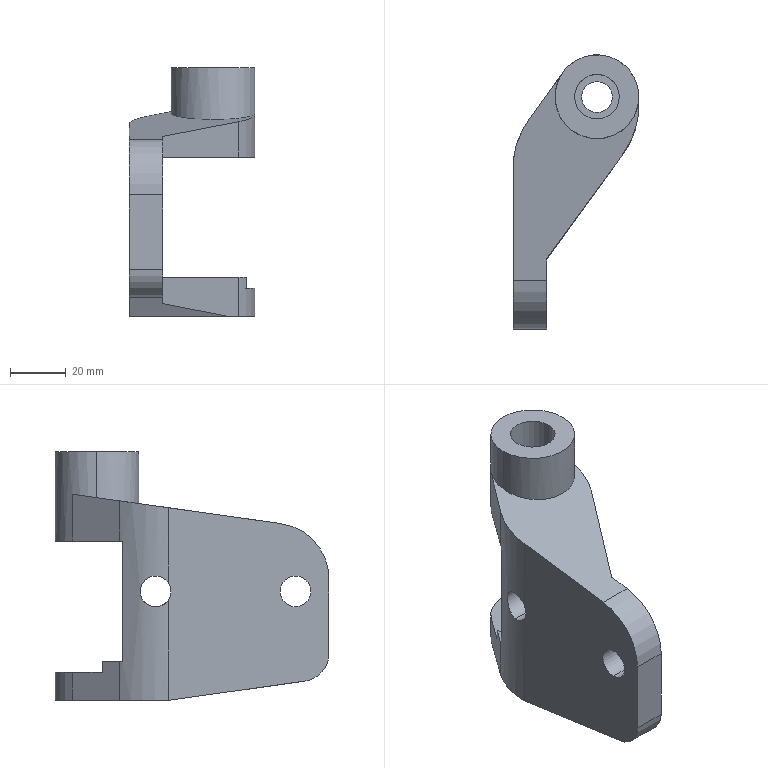Part | SolidWorks | features BaseBody 1 | 1 solid | 40 faces | box 45 x 98 x 89 mm | volume 93140 mm3 | cylinder 21 | plane 19 | commonest cylinder face diameters 11 x6 20 x5 30 x3 60 x3 16 x2 40 x2
STEP:
#1=CARTESIAN_POINT('',(-30.,-71.,33.5));
#2=VERTEX_POINT('',#1);
#3=CARTESIAN_POINT('',(-30.,-71.,44.5));
#4=VERTEX_POINT('',#3);
#5=CARTESIAN_POINT('',(-30.,-71.,39.));
#6=DIRECTION('',(-1.,0.,0.));
#7=DIRECTION('',(0.,0.,-1.));
#8=AXIS2_PLACEMENT_3D('',#5,#6,#7);
#9=CIRCLE('',#8,5.5);
#10=EDGE_CURVE('',#2,#4,#9,.T.);
#11=ORIENTED_EDGE('',*,*,#10,.T.);
#12=CARTESIAN_POINT('',(-19.,-71.,44.5));
#13=VERTEX_POINT('',#12);
#14=CARTESIAN_POINT('',(-30.,-71.,44.5));
#15=DIRECTION('',(1.,0.,0.));
#16=VECTOR('',#15,1000.);
#17=LINE('',#14,#16);
#18=EDGE_CURVE('',#4,#13,#17,.T.);
#19=ORIENTED_EDGE('',*,*,#18,.T.);
#20=CARTESIAN_POINT('',(-19.,-71.,33.5));
#21=VERTEX_POINT('',#20);
#22=CARTESIAN_POINT('',(-19.,-71.,39.));
#23=DIRECTION('',(-1.,0.,0.));
#24=DIRECTION('',(0.,0.,-1.));
#25=AXIS2_PLACEMENT_3D('',#22,#23,#24);
#26=CIRCLE('',#25,5.5);
#27=EDGE_CURVE('',#21,#13,#26,.T.);
#28=ORIENTED_EDGE('',*,*,#27,.F.);
#29=CARTESIAN_POINT('',(-30.,-71.,33.5));
#30=DIRECTION('',(1.,0.,0.));
#31=VECTOR('',#30,1000.);
#32=LINE('',#29,#31);
#33=EDGE_CURVE('',#2,#21,#32,.T.);
#34=ORIENTED_EDGE('',*,*,#33,.F.);
#35=EDGE_LOOP('',(#11,#19,#28,#34));
#36=FACE_OUTER_BOUND('',#35,.T.);
#37=CARTESIAN_POINT('',(-30.,-71.,39.));
#38=DIRECTION('',(1.,0.,0.));
#39=DIRECTION('',(0.,0.,-1.));
#40=AXIS2_PLACEMENT_3D('',#37,#38,#39);
#41=CYLINDRICAL_SURFACE('',#40,5.5);
#42=ADVANCED_FACE('',(#36),#41,.F.);
#43=CARTESIAN_POINT('',(-29.641,-21.,44.5));
#44=VERTEX_POINT('',#43);
#45=CARTESIAN_POINT('',(-30.,-25.63,41.969));
#46=VERTEX_POINT('',#45);
#47=CARTESIAN_POINT('',(-29.641,-21.,44.5));
#48=CARTESIAN_POINT('',(-29.676,-21.226,44.5));
#49=CARTESIAN_POINT('',(-29.709,-21.456,44.486));
#50=CARTESIAN_POINT('',(-29.769,-21.91,44.429));
#51=CARTESIAN_POINT('',(-29.796,-22.134,44.387));
#52=CARTESIAN_POINT('',(-29.845,-22.574,44.275));
#53=CARTESIAN_POINT('',(-29.866,-22.791,44.205));
#54=CARTESIAN_POINT('',(-29.904,-23.218,44.038));
#55=CARTESIAN_POINT('',(-29.92,-23.429,43.94));
#56=CARTESIAN_POINT('',(-29.96,-24.033,43.611));
#57=CARTESIAN_POINT('',(-29.977,-24.405,43.344));
#58=CARTESIAN_POINT('',(-29.997,-25.082,42.715));
#59=CARTESIAN_POINT('',(-30.,-25.379,42.36));
#60=CARTESIAN_POINT('',(-30.,-25.63,41.969));
#61=B_SPLINE_CURVE_WITH_KNOTS('',3,(#47,#48,#49,#50,#51,#52,#53,#54,#55,#56,#57,#58,#59,#60),.UNSPECIFIED.,.F.,.F.,(4,2,2,2,2,2,4),(0.008728,0.009414,0.0101,0.01079,0.01147,0.01284,0.01422),.UNSPECIFIED.);
#62=EDGE_CURVE('',#44,#46,#61,.T.);
#63=ORIENTED_EDGE('',*,*,#62,.F.);
#64=CARTESIAN_POINT('',(-19.,-21.,44.5));
#65=VERTEX_POINT('',#64);
#66=CARTESIAN_POINT('',(-30.,-21.,44.5));
#67=DIRECTION('',(1.,0.,0.));
#68=VECTOR('',#67,1000.);
#69=LINE('',#66,#68);
#70=EDGE_CURVE('',#44,#65,#69,.T.);
#71=ORIENTED_EDGE('',*,*,#70,.T.);
#72=CARTESIAN_POINT('',(-19.,-21.,33.5));
#73=VERTEX_POINT('',#72);
#74=CARTESIAN_POINT('',(-19.,-21.,39.));
#75=DIRECTION('',(-1.,0.,0.));
#76=DIRECTION('',(0.,0.,-1.));
#77=AXIS2_PLACEMENT_3D('',#74,#75,#76);
#78=CIRCLE('',#77,5.5);
#79=EDGE_CURVE('',#73,#65,#78,.T.);
#80=ORIENTED_EDGE('',*,*,#79,.F.);
#81=CARTESIAN_POINT('',(-29.641,-21.,33.5));
#82=VERTEX_POINT('',#81);
#83=CARTESIAN_POINT('',(-30.,-21.,33.5));
#84=DIRECTION('',(1.,0.,0.));
#85=VECTOR('',#84,1000.);
#86=LINE('',#83,#85);
#87=EDGE_CURVE('',#82,#73,#86,.T.);
#88=ORIENTED_EDGE('',*,*,#87,.F.);
#89=CARTESIAN_POINT('',(-30.,-25.63,36.031));
#90=VERTEX_POINT('',#89);
#91=CARTESIAN_POINT('',(-30.,-25.63,36.031));
#92=CARTESIAN_POINT('',(-30.,-25.379,35.64));
#93=CARTESIAN_POINT('',(-29.997,-25.085,35.289));
#94=CARTESIAN_POINT('',(-29.982,-24.581,34.819));
#95=CARTESIAN_POINT('',(-29.975,-24.401,34.671));
#96=CARTESIAN_POINT('',(-29.958,-24.026,34.402));
#97=CARTESIAN_POINT('',(-29.947,-23.832,34.28));
#98=CARTESIAN_POINT('',(-29.92,-23.431,34.061));
#99=CARTESIAN_POINT('',(-29.904,-23.223,33.964));
#100=CARTESIAN_POINT('',(-29.867,-22.795,33.796));
#101=CARTESIAN_POINT('',(-29.845,-22.574,33.725));
#102=CARTESIAN_POINT('',(-29.772,-21.91,33.557));
#103=CARTESIAN_POINT('',(-29.712,-21.459,33.5));
#104=CARTESIAN_POINT('',(-29.641,-21.,33.5));
#105=B_SPLINE_CURVE_WITH_KNOTS('',3,(#91,#92,#93,#94,#95,#96,#97,#98,#99,#100,#101,#102,#103,#104),.UNSPECIFIED.,.F.,.F.,(4,2,2,2,2,2,4),(-0.01422,-0.01284,-0.01216,-0.01147,-0.01078,-0.0101,-0.008723),.UNSPECIFIED.);
#106=EDGE_CURVE('',#90,#82,#105,.T.);
#107=ORIENTED_EDGE('',*,*,#106,.F.);
#108=CARTESIAN_POINT('',(-30.,-21.,39.));
#109=DIRECTION('',(-1.,0.,0.));
#110=DIRECTION('',(0.,0.,-1.));
#111=AXIS2_PLACEMENT_3D('',#108,#109,#110);
#112=CIRCLE('',#111,5.5);
#113=EDGE_CURVE('',#90,#46,#112,.T.);
#114=ORIENTED_EDGE('',*,*,#113,.T.);
#115=EDGE_LOOP('',(#63,#71,#80,#88,#107,#114));
#116=FACE_OUTER_BOUND('',#115,.T.);
#117=CARTESIAN_POINT('',(-30.,-21.,39.));
#118=DIRECTION('',(1.,0.,0.));
#119=DIRECTION('',(0.,0.,-1.));
#120=AXIS2_PLACEMENT_3D('',#117,#118,#119);
#121=CYLINDRICAL_SURFACE('',#120,5.5);
#122=ADVANCED_FACE('',(#116),#121,.F.);
#123=CARTESIAN_POINT('',(-15.,0.,89.));
#124=VERTEX_POINT('',#123);
#125=CARTESIAN_POINT('',(15.,0.,89.));
#126=VERTEX_POINT('',#125);
#127=CARTESIAN_POINT('',(0.,0.,89.));
#128=DIRECTION('',(0.,0.,-1.));
#129=DIRECTION('',(-1.,0.,0.));
#130=AXIS2_PLACEMENT_3D('',#127,#128,#129);
#131=CIRCLE('',#130,15.);
#132=EDGE_CURVE('',#124,#126,#131,.T.);
#133=ORIENTED_EDGE('',*,*,#132,.T.);
#134=CARTESIAN_POINT('',(15.,-0.000000405,72.514));
#135=VERTEX_POINT('',#134);
#136=CARTESIAN_POINT('',(15.,0.,89.));
#137=DIRECTION('',(0.,0.,-1.));
#138=VECTOR('',#137,1000.);
#139=LINE('',#136,#138);
#140=EDGE_CURVE('',#126,#135,#139,.T.);
#141=ORIENTED_EDGE('',*,*,#140,.T.);
#142=CARTESIAN_POINT('',(15.,-0.000000405,57.));
#143=VERTEX_POINT('',#142);
#144=CARTESIAN_POINT('',(15.,-0.00000081,89.));
#145=DIRECTION('',(0.,0.,-1.));
#146=VECTOR('',#145,1000.);
#147=LINE('',#144,#146);
#148=EDGE_CURVE('',#135,#143,#147,.T.);
#149=ORIENTED_EDGE('',*,*,#148,.T.);
#150=CARTESIAN_POINT('',(-12.163,8.779,57.));
#151=VERTEX_POINT('',#150);
#152=CARTESIAN_POINT('',(0.,0.,57.));
#153=DIRECTION('',(0.,0.,1.));
#154=DIRECTION('',(-1.,0.,0.));
#155=AXIS2_PLACEMENT_3D('',#152,#153,#154);
#156=CIRCLE('',#155,15.);
#157=EDGE_CURVE('',#143,#151,#156,.T.);
#158=ORIENTED_EDGE('',*,*,#157,.T.);
#159=CARTESIAN_POINT('',(-12.163,8.779,73.747));
#160=VERTEX_POINT('',#159);
#161=CARTESIAN_POINT('',(-12.163,8.779,65.374));
#162=DIRECTION('',(0.,0.,1.));
#163=VECTOR('',#162,1000.);
#164=LINE('',#161,#163);
#165=EDGE_CURVE('',#151,#160,#164,.T.);
#166=ORIENTED_EDGE('',*,*,#165,.T.);
#167=CARTESIAN_POINT('',(-15.,0.,72.514));
#168=VERTEX_POINT('',#167);
#169=CARTESIAN_POINT('',(-15.,0.,72.514));
#170=CARTESIAN_POINT('',(-15.,3.178,72.96));
#171=CARTESIAN_POINT('',(-14.023,6.202,73.385));
#172=CARTESIAN_POINT('',(-12.163,8.779,73.747));
#173=(BOUNDED_CURVE()B_SPLINE_CURVE(3,(#169,#170,#171,#172),.UNSPECIFIED.,.F.,.F.)B_SPLINE_CURVE_WITH_KNOTS((4,4),(1.571,2.196),.UNSPECIFIED.)CURVE()GEOMETRIC_REPRESENTATION_ITEM()RATIONAL_B_SPLINE_CURVE((1.,0.9677,0.9677,1.))REPRESENTATION_ITEM(''));
#174=EDGE_CURVE('',#168,#160,#173,.T.);
#175=ORIENTED_EDGE('',*,*,#174,.F.);
#176=CARTESIAN_POINT('',(-15.,0.,89.));
#177=DIRECTION('',(0.,0.,-1.));
#178=VECTOR('',#177,1000.);
#179=LINE('',#176,#178);
#180=EDGE_CURVE('',#124,#168,#179,.T.);
#181=ORIENTED_EDGE('',*,*,#180,.F.);
#182=EDGE_LOOP('',(#133,#141,#149,#158,#166,#175,#181));
#183=FACE_OUTER_BOUND('',#182,.T.);
#184=CARTESIAN_POINT('',(0.,0.,89.));
#185=DIRECTION('',(0.,0.,-1.));
#186=DIRECTION('',(-1.,0.,0.));
#187=AXIS2_PLACEMENT_3D('',#184,#185,#186);
#188=CYLINDRICAL_SURFACE('',#187,15.);
#189=ADVANCED_FACE('',(#183),#188,.T.);
#190=CARTESIAN_POINT('',(-18.,-71.,29.));
#191=VERTEX_POINT('',#190);
#192=CARTESIAN_POINT('',(-18.,-71.,49.));
#193=VERTEX_POINT('',#192);
#194=CARTESIAN_POINT('',(-18.,-71.,39.));
#195=DIRECTION('',(-1.,0.,0.));
#196=DIRECTION('',(0.,0.,1.));
#197=AXIS2_PLACEMENT_3D('',#194,#195,#196);
#198=CIRCLE('',#197,10.);
#199=EDGE_CURVE('',#191,#193,#198,.T.);
#200=ORIENTED_EDGE('',*,*,#199,.F.);
#201=CARTESIAN_POINT('',(-19.,-71.,29.));
#202=VERTEX_POINT('',#201);
#203=CARTESIAN_POINT('',(-18.,-71.,29.));
#204=DIRECTION('',(-1.,0.,0.));
#205=VECTOR('',#204,1000.);
#206=LINE('',#203,#205);
#207=EDGE_CURVE('',#191,#202,#206,.T.);
#208=ORIENTED_EDGE('',*,*,#207,.T.);
#209=CARTESIAN_POINT('',(-19.,-71.,49.));
#210=VERTEX_POINT('',#209);
#211=CARTESIAN_POINT('',(-19.,-71.,39.));
#212=DIRECTION('',(1.,0.,0.));
#213=DIRECTION('',(0.,0.,1.));
#214=AXIS2_PLACEMENT_3D('',#211,#212,#213);
#215=CIRCLE('',#214,10.);
#216=EDGE_CURVE('',#210,#202,#215,.T.);
#217=ORIENTED_EDGE('',*,*,#216,.F.);
#218=CARTESIAN_POINT('',(-18.,-71.,49.));
#219=DIRECTION('',(-1.,0.,0.));
#220=VECTOR('',#219,1000.);
#221=LINE('',#218,#220);
#222=EDGE_CURVE('',#193,#210,#221,.T.);
#223=ORIENTED_EDGE('',*,*,#222,.F.);
#224=EDGE_LOOP('',(#200,#208,#217,#223));
#225=FACE_OUTER_BOUND('',#224,.T.);
#226=CARTESIAN_POINT('',(-18.,-71.,39.));
#227=DIRECTION('',(-1.,0.,0.));
#228=DIRECTION('',(0.,0.,1.));
#229=AXIS2_PLACEMENT_3D('',#226,#227,#228);
#230=CYLINDRICAL_SURFACE('',#229,10.);
#231=ADVANCED_FACE('',(#225),#230,.F.);
#232=CARTESIAN_POINT('',(-18.,-21.,29.));
#233=VERTEX_POINT('',#232);
#234=CARTESIAN_POINT('',(-18.,-21.,49.));
#235=VERTEX_POINT('',#234);
#236=CARTESIAN_POINT('',(-18.,-21.,39.));
#237=DIRECTION('',(-1.,0.,0.));
#238=DIRECTION('',(0.,0.,1.));
#239=AXIS2_PLACEMENT_3D('',#236,#237,#238);
#240=CIRCLE('',#239,10.);
#241=EDGE_CURVE('',#233,#235,#240,.T.);
#242=ORIENTED_EDGE('',*,*,#241,.F.);
#243=CARTESIAN_POINT('',(-19.,-21.,29.));
#244=VERTEX_POINT('',#243);
#245=CARTESIAN_POINT('',(-18.,-21.,29.));
#246=DIRECTION('',(-1.,0.,0.));
#247=VECTOR('',#246,1000.);
#248=LINE('',#245,#247);
#249=EDGE_CURVE('',#233,#244,#248,.T.);
#250=ORIENTED_EDGE('',*,*,#249,.T.);
#251=CARTESIAN_POINT('',(-19.,-21.,49.));
#252=VERTEX_POINT('',#251);
#253=CARTESIAN_POINT('',(-19.,-21.,39.));
#254=DIRECTION('',(1.,0.,0.));
#255=DIRECTION('',(0.,0.,1.));
#256=AXIS2_PLACEMENT_3D('',#253,#254,#255);
#257=CIRCLE('',#256,10.);
#258=EDGE_CURVE('',#252,#244,#257,.T.);
#259=ORIENTED_EDGE('',*,*,#258,.F.);
#260=CARTESIAN_POINT('',(-18.,-21.,49.));
#261=DIRECTION('',(-1.,0.,0.));
#262=VECTOR('',#261,1000.);
#263=LINE('',#260,#262);
#264=EDGE_CURVE('',#235,#252,#263,.T.);
#265=ORIENTED_EDGE('',*,*,#264,.F.);
#266=EDGE_LOOP('',(#242,#250,#259,#265));
#267=FACE_OUTER_BOUND('',#266,.T.);
#268=CARTESIAN_POINT('',(-18.,-21.,39.));
#269=DIRECTION('',(-1.,0.,0.));
#270=DIRECTION('',(0.,0.,1.));
#271=AXIS2_PLACEMENT_3D('',#268,#269,#270);
#272=CYLINDRICAL_SURFACE('',#271,10.);
#273=ADVANCED_FACE('',(#267),#272,.F.);
#274=CARTESIAN_POINT('',(5.5,0.,0.));
#275=VERTEX_POINT('',#274);
#276=CARTESIAN_POINT('',(-5.5,0.,0.));
#277=VERTEX_POINT('',#276);
#278=CARTESIAN_POINT('',(0.,0.,0.));
#279=DIRECTION('',(0.,0.,-1.));
#280=DIRECTION('',(1.,0.,0.));
#281=AXIS2_PLACEMENT_3D('',#278,#279,#280);
#282=CIRCLE('',#281,5.5);
#283=EDGE_CURVE('',#275,#277,#282,.T.);
#284=ORIENTED_EDGE('',*,*,#283,.T.);
#285=CARTESIAN_POINT('',(-5.5,0.,10.));
#286=VERTEX_POINT('',#285);
#287=CARTESIAN_POINT('',(-5.5,0.,0.));
#288=DIRECTION('',(0.,0.,1.));
#289=VECTOR('',#288,1000.);
#290=LINE('',#287,#289);
#291=EDGE_CURVE('',#277,#286,#290,.T.);
#292=ORIENTED_EDGE('',*,*,#291,.T.);
#293=CARTESIAN_POINT('',(5.5,0.,10.));
#294=VERTEX_POINT('',#293);
#295=CARTESIAN_POINT('',(0.,0.,10.));
#296=DIRECTION('',(0.,0.,-1.));
#297=DIRECTION('',(1.,0.,0.));
#298=AXIS2_PLACEMENT_3D('',#295,#296,#297);
#299=CIRCLE('',#298,5.5);
#300=EDGE_CURVE('',#294,#286,#299,.T.);
#301=ORIENTED_EDGE('',*,*,#300,.F.);
#302=CARTESIAN_POINT('',(5.5,0.,0.));
#303=DIRECTION('',(0.,0.,1.));
#304=VECTOR('',#303,1000.);
#305=LINE('',#302,#304);
#306=EDGE_CURVE('',#275,#294,#305,.T.);
#307=ORIENTED_EDGE('',*,*,#306,.F.);
#308=EDGE_LOOP('',(#284,#292,#301,#307));
#309=FACE_OUTER_BOUND('',#308,.T.);
#310=CARTESIAN_POINT('',(0.,0.,0.));
#311=DIRECTION('',(0.,0.,1.));
#312=DIRECTION('',(1.,0.,0.));
#313=AXIS2_PLACEMENT_3D('',#310,#311,#312);
#314=CYLINDRICAL_SURFACE('',#313,5.5);
#315=ADVANCED_FACE('',(#309),#314,.F.);
#316=CARTESIAN_POINT('',(8.,0.,89.));
#317=VERTEX_POINT('',#316);
#318=CARTESIAN_POINT('',(-8.,0.,89.));
#319=VERTEX_POINT('',#318);
#320=CARTESIAN_POINT('',(0.,0.,89.));
#321=DIRECTION('',(0.,0.,-1.));
#322=DIRECTION('',(-1.,0.,0.));
#323=AXIS2_PLACEMENT_3D('',#320,#321,#322);
#324=CIRCLE('',#323,8.);
#325=EDGE_CURVE('',#317,#319,#324,.T.);
#326=ORIENTED_EDGE('',*,*,#325,.F.);
#327=CARTESIAN_POINT('',(8.,0.,57.));
#328=VERTEX_POINT('',#327);
#329=CARTESIAN_POINT('',(8.,0.,89.));
#330=DIRECTION('',(0.,0.,-1.));
#331=VECTOR('',#330,1000.);
#332=LINE('',#329,#331);
#333=EDGE_CURVE('',#317,#328,#332,.T.);
#334=ORIENTED_EDGE('',*,*,#333,.T.);
#335=CARTESIAN_POINT('',(-8.,0.,57.));
#336=VERTEX_POINT('',#335);
#337=CARTESIAN_POINT('',(0.,0.,57.));
#338=DIRECTION('',(0.,0.,-1.));
#339=DIRECTION('',(-1.,0.,0.));
#340=AXIS2_PLACEMENT_3D('',#337,#338,#339);
#341=CIRCLE('',#340,8.);
#342=EDGE_CURVE('',#328,#336,#341,.T.);
#343=ORIENTED_EDGE('',*,*,#342,.T.);
#344=CARTESIAN_POINT('',(-8.,0.,89.));
#345=DIRECTION('',(0.,0.,-1.));
#346=VECTOR('',#345,1000.);
#347=LINE('',#344,#346);
#348=EDGE_CURVE('',#319,#336,#347,.T.);
#349=ORIENTED_EDGE('',*,*,#348,.F.);
#350=EDGE_LOOP('',(#326,#334,#343,#349));
#351=FACE_OUTER_BOUND('',#350,.T.);
#352=CARTESIAN_POINT('',(0.,0.,89.));
#353=DIRECTION('',(0.,0.,-1.));
#354=DIRECTION('',(-1.,0.,0.));
#355=AXIS2_PLACEMENT_3D('',#352,#353,#354);
#356=CYLINDRICAL_SURFACE('',#355,8.);
#357=ADVANCED_FACE('',(#351),#356,.F.);
#358=ORIENTED_EDGE('',*,*,#10,.F.);
#359=CARTESIAN_POINT('',(-30.,-71.,39.));
#360=DIRECTION('',(-1.,0.,0.));
#361=DIRECTION('',(0.,0.,-1.));
#362=AXIS2_PLACEMENT_3D('',#359,#360,#361);
#363=CIRCLE('',#362,5.5);
#364=EDGE_CURVE('',#4,#2,#363,.T.);
#365=ORIENTED_EDGE('',*,*,#364,.F.);
#366=EDGE_LOOP('',(#358,#365));
#367=FACE_BOUND('',#366,.T.);
#368=CARTESIAN_POINT('',(-30.,-25.63,68.911));
#369=VERTEX_POINT('',#368);
#370=CARTESIAN_POINT('',(-30.,-65.783,63.268));
#371=VERTEX_POINT('',#370);
#372=CARTESIAN_POINT('',(-30.,-25.63,68.911));
#373=DIRECTION('',(0.,-0.9903,-0.1392));
#374=VECTOR('',#373,1000.);
#375=LINE('',#372,#374);
#376=EDGE_CURVE('',#369,#371,#375,.T.);
#377=ORIENTED_EDGE('',*,*,#376,.F.);
#378=CARTESIAN_POINT('',(-30.,-25.63,34.475));
#379=DIRECTION('',(0.,0.,1.));
#380=VECTOR('',#379,1000.);
#381=LINE('',#378,#380);
#382=EDGE_CURVE('',#46,#369,#381,.T.);
#383=ORIENTED_EDGE('',*,*,#382,.F.);
#384=ORIENTED_EDGE('',*,*,#113,.F.);
#385=CARTESIAN_POINT('',(-30.,-25.63,0.03827));
#386=VERTEX_POINT('',#385);
#387=CARTESIAN_POINT('',(-30.,-25.63,34.475));
#388=DIRECTION('',(0.,0.,1.));
#389=VECTOR('',#388,1000.);
#390=LINE('',#387,#389);
#391=EDGE_CURVE('',#386,#90,#390,.T.);
#392=ORIENTED_EDGE('',*,*,#391,.F.);
#393=CARTESIAN_POINT('',(-30.,-74.392,6.891));
#394=VERTEX_POINT('',#393);
#395=CARTESIAN_POINT('',(-30.,-74.392,6.891));
#396=DIRECTION('',(0.,0.9903,-0.1392));
#397=VECTOR('',#396,1000.);
#398=LINE('',#395,#397);
#399=EDGE_CURVE('',#394,#386,#398,.T.);
#400=ORIENTED_EDGE('',*,*,#399,.F.);
#401=CARTESIAN_POINT('',(-30.,-83.,16.794));
#402=VERTEX_POINT('',#401);
#403=CARTESIAN_POINT('',(-30.,-73.,16.794));
#404=DIRECTION('',(1.,0.,0.));
#405=DIRECTION('',(0.,0.,1.));
#406=AXIS2_PLACEMENT_3D('',#403,#404,#405);
#407=CIRCLE('',#406,10.);
#408=EDGE_CURVE('',#402,#394,#407,.T.);
#409=ORIENTED_EDGE('',*,*,#408,.F.);
#410=CARTESIAN_POINT('',(-30.,-83.,43.463));
#411=VERTEX_POINT('',#410);
#412=CARTESIAN_POINT('',(-30.,-83.,34.475));
#413=DIRECTION('',(0.,0.,-1.));
#414=VECTOR('',#413,1000.);
#415=LINE('',#412,#414);
#416=EDGE_CURVE('',#411,#402,#415,.T.);
#417=ORIENTED_EDGE('',*,*,#416,.F.);
#418=CARTESIAN_POINT('',(-30.,-63.,43.463));
#419=DIRECTION('',(1.,0.,0.));
#420=DIRECTION('',(0.,0.,1.));
#421=AXIS2_PLACEMENT_3D('',#418,#419,#420);
#422=CIRCLE('',#421,20.);
#423=EDGE_CURVE('',#371,#411,#422,.T.);
#424=ORIENTED_EDGE('',*,*,#423,.F.);
#425=EDGE_LOOP('',(#377,#383,#384,#392,#400,#409,#417,#424));
#426=FACE_OUTER_BOUND('',#425,.T.);
#427=CARTESIAN_POINT('',(-30.,-54.315,34.475));
#428=DIRECTION('',(1.,0.,0.));
#429=DIRECTION('',(0.,0.,-1.));
#430=AXIS2_PLACEMENT_3D('',#427,#428,#429);
#431=PLANE('',#430);
#432=ADVANCED_FACE('',(#367,#426),#431,.F.);
#433=ORIENTED_EDGE('',*,*,#18,.F.);
#434=ORIENTED_EDGE('',*,*,#364,.T.);
#435=ORIENTED_EDGE('',*,*,#33,.T.);
#436=CARTESIAN_POINT('',(-19.,-71.,39.));
#437=DIRECTION('',(-1.,0.,0.));
#438=DIRECTION('',(0.,0.,-1.));
#439=AXIS2_PLACEMENT_3D('',#436,#437,#438);
#440=CIRCLE('',#439,5.5);
#441=EDGE_CURVE('',#13,#21,#440,.T.);
#442=ORIENTED_EDGE('',*,*,#441,.F.);
#443=EDGE_LOOP('',(#433,#434,#435,#442));
#444=FACE_OUTER_BOUND('',#443,.T.);
#445=CARTESIAN_POINT('',(-30.,-71.,39.));
#446=DIRECTION('',(1.,0.,0.));
#447=DIRECTION('',(0.,0.,-1.));
#448=AXIS2_PLACEMENT_3D('',#445,#446,#447);
#449=CYLINDRICAL_SURFACE('',#448,5.5);
#450=ADVANCED_FACE('',(#444),#449,.F.);
#451=CARTESIAN_POINT('',(-18.,-83.,43.463));
#452=VERTEX_POINT('',#451);
#453=CARTESIAN_POINT('',(-18.,-83.,43.463));
#454=DIRECTION('',(1.,0.,0.));
#455=VECTOR('',#454,1000.);
#456=LINE('',#453,#455);
#457=EDGE_CURVE('',#411,#452,#456,.T.);
#458=ORIENTED_EDGE('',*,*,#457,.T.);
#459=CARTESIAN_POINT('',(-18.,-65.783,63.268));
#460=VERTEX_POINT('',#459);
#461=CARTESIAN_POINT('',(-18.,-63.,43.463));
#462=DIRECTION('',(-1.,0.,0.));
#463=DIRECTION('',(0.,0.,1.));
#464=AXIS2_PLACEMENT_3D('',#461,#462,#463);
#465=CIRCLE('',#464,20.);
#466=EDGE_CURVE('',#452,#460,#465,.T.);
#467=ORIENTED_EDGE('',*,*,#466,.T.);
#468=CARTESIAN_POINT('',(-18.,-65.783,63.268));
#469=DIRECTION('',(-1.,0.,0.));
#470=VECTOR('',#469,1000.);
#471=LINE('',#468,#470);
#472=EDGE_CURVE('',#460,#371,#471,.T.);
#473=ORIENTED_EDGE('',*,*,#472,.T.);
#474=ORIENTED_EDGE('',*,*,#423,.T.);
#475=EDGE_LOOP('',(#458,#467,#473,#474));
#476=FACE_OUTER_BOUND('',#475,.T.);
#477=CARTESIAN_POINT('',(-18.,-63.,43.463));
#478=DIRECTION('',(-1.,0.,0.));
#479=DIRECTION('',(0.,0.,1.));
#480=AXIS2_PLACEMENT_3D('',#477,#478,#479);
#481=CYLINDRICAL_SURFACE('',#480,20.);
#482=ADVANCED_FACE('',(#476),#481,.T.);
#483=CARTESIAN_POINT('',(15.,-0.000000405,72.514));
#484=CARTESIAN_POINT('',(15.,-30.,68.297));
#485=CARTESIAN_POINT('',(-15.,-30.,68.297));
#486=CARTESIAN_POINT('',(-15.,0.,72.514));
#487=(BOUNDED_CURVE()B_SPLINE_CURVE(3,(#483,#484,#485,#486),.UNSPECIFIED.,.F.,.F.)B_SPLINE_CURVE_WITH_KNOTS((4,4),(4.712,7.854),.UNSPECIFIED.)CURVE()GEOMETRIC_REPRESENTATION_ITEM()RATIONAL_B_SPLINE_CURVE((1.,0.3333,0.3333,1.))REPRESENTATION_ITEM(''));
#488=EDGE_CURVE('',#135,#168,#487,.T.);
#489=ORIENTED_EDGE('',*,*,#488,.T.);
#490=ORIENTED_EDGE('',*,*,#174,.T.);
#491=CARTESIAN_POINT('',(-24.325,-8.072,71.379));
#492=VERTEX_POINT('',#491);
#493=CARTESIAN_POINT('',(-12.163,8.779,73.747));
#494=DIRECTION('',(-0.5815,-0.8056,-0.1132));
#495=VECTOR('',#494,1000.);
#496=LINE('',#493,#495);
#497=EDGE_CURVE('',#160,#492,#496,.T.);
#498=ORIENTED_EDGE('',*,*,#497,.T.);
#499=CARTESIAN_POINT('',(-24.325,-8.072,71.379));
#500=CARTESIAN_POINT('',(-28.045,-13.226,70.655));
#501=CARTESIAN_POINT('',(-30.,-19.274,69.805));
#502=CARTESIAN_POINT('',(-30.,-25.63,68.911));
#503=(BOUNDED_CURVE()B_SPLINE_CURVE(3,(#499,#500,#501,#502),.UNSPECIFIED.,.F.,.F.)B_SPLINE_CURVE_WITH_KNOTS((4,4),(4.087,4.712),.UNSPECIFIED.)CURVE()GEOMETRIC_REPRESENTATION_ITEM()RATIONAL_B_SPLINE_CURVE((1.,0.9677,0.9677,1.))REPRESENTATION_ITEM(''));
#504=EDGE_CURVE('',#492,#369,#503,.T.);
#505=ORIENTED_EDGE('',*,*,#504,.T.);
#506=ORIENTED_EDGE('',*,*,#376,.T.);
#507=ORIENTED_EDGE('',*,*,#472,.F.);
#508=CARTESIAN_POINT('',(-18.,-58.,64.362));
#509=VERTEX_POINT('',#508);
#510=CARTESIAN_POINT('',(-18.,-28.502,68.508));
#511=DIRECTION('',(0.,0.9903,0.1392));
#512=VECTOR('',#511,1000.);
#513=LINE('',#510,#512);
#514=EDGE_CURVE('',#460,#509,#513,.T.);
#515=ORIENTED_EDGE('',*,*,#514,.T.);
#516=CARTESIAN_POINT('',(9.271,-20.465,69.637));
#517=VERTEX_POINT('',#516);
#518=CARTESIAN_POINT('',(-18.,-58.,64.362));
#519=DIRECTION('',(0.584,0.8038,0.113));
#520=VECTOR('',#519,1000.);
#521=LINE('',#518,#520);
#522=EDGE_CURVE('',#509,#517,#521,.T.);
#523=ORIENTED_EDGE('',*,*,#522,.T.);
#524=CARTESIAN_POINT('',(15.,-2.832,72.116));
#525=VERTEX_POINT('',#524);
#526=CARTESIAN_POINT('',(9.271,-20.465,69.637));
#527=CARTESIAN_POINT('',(13.026,-15.297,70.364));
#528=CARTESIAN_POINT('',(15.,-9.221,71.218));
#529=CARTESIAN_POINT('',(15.,-2.832,72.116));
#530=(BOUNDED_CURVE()B_SPLINE_CURVE(3,(#526,#527,#528,#529),.UNSPECIFIED.,.F.,.T.)B_SPLINE_CURVE_WITH_KNOTS((4,4),(0.9425,1.571),.UNSPECIFIED.)CURVE()GEOMETRIC_REPRESENTATION_ITEM()RATIONAL_B_SPLINE_CURVE((1.,0.9674,0.9674,1.))REPRESENTATION_ITEM(''));
#531=EDGE_CURVE('',#517,#525,#530,.T.);
#532=ORIENTED_EDGE('',*,*,#531,.T.);
#533=CARTESIAN_POINT('',(15.,-28.502,68.508));
#534=DIRECTION('',(0.,0.9903,0.1392));
#535=VECTOR('',#534,1000.);
#536=LINE('',#533,#535);
#537=EDGE_CURVE('',#525,#135,#536,.T.);
#538=ORIENTED_EDGE('',*,*,#537,.T.);
#539=EDGE_LOOP('',(#489,#490,#498,#505,#506,#507,#515,#523,#532,#538));
#540=FACE_OUTER_BOUND('',#539,.T.);
#541=CARTESIAN_POINT('',(-7.5,-28.502,68.508));
#542=DIRECTION('',(0.,-0.1392,0.9903));
#543=DIRECTION('',(0.,-0.9903,-0.1392));
#544=AXIS2_PLACEMENT_3D('',#541,#542,#543);
#545=PLANE('',#544);
#546=ADVANCED_FACE('',(#540),#545,.T.);
#547=ORIENTED_EDGE('',*,*,#391,.T.);
#548=ORIENTED_EDGE('',*,*,#106,.T.);
#549=CARTESIAN_POINT('',(-29.641,-21.,33.5));
#550=CARTESIAN_POINT('',(-29.584,-20.636,33.5));
#551=CARTESIAN_POINT('',(-29.521,-20.278,33.536));
#552=CARTESIAN_POINT('',(-29.419,-19.752,33.64));
#553=CARTESIAN_POINT('',(-29.384,-19.579,33.684));
#554=CARTESIAN_POINT('',(-29.311,-19.235,33.788));
#555=CARTESIAN_POINT('',(-29.273,-19.064,33.849));
#556=CARTESIAN_POINT('',(-29.159,-18.569,34.054));
#557=CARTESIAN_POINT('',(-29.081,-18.255,34.221));
#558=CARTESIAN_POINT('',(-28.924,-17.661,34.615));
#559=CARTESIAN_POINT('',(-28.845,-17.38,34.844));
#560=CARTESIAN_POINT('',(-28.695,-16.874,35.345));
#561=CARTESIAN_POINT('',(-28.624,-16.646,35.62));
#562=CARTESIAN_POINT('',(-28.527,-16.343,36.068));
#563=CARTESIAN_POINT('',(-28.496,-16.249,36.224));
#564=CARTESIAN_POINT('',(-28.439,-16.077,36.541));
#565=CARTESIAN_POINT('',(-28.412,-15.999,36.704));
#566=CARTESIAN_POINT('',(-28.341,-15.79,37.201));
#567=CARTESIAN_POINT('',(-28.303,-15.682,37.549));
#568=CARTESIAN_POINT('',(-28.251,-15.536,38.269));
#569=CARTESIAN_POINT('',(-28.238,-15.5,38.634));
#570=CARTESIAN_POINT('',(-28.238,-15.5,39.372));
#571=CARTESIAN_POINT('',(-28.251,-15.537,39.734));
#572=CARTESIAN_POINT('',(-28.302,-15.681,40.445));
#573=CARTESIAN_POINT('',(-28.341,-15.79,40.798));
#574=CARTESIAN_POINT('',(-28.437,-16.071,41.466));
#575=CARTESIAN_POINT('',(-28.494,-16.242,41.782));
#576=CARTESIAN_POINT('',(-28.591,-16.545,42.23));
#577=CARTESIAN_POINT('',(-28.626,-16.654,42.375));
#578=CARTESIAN_POINT('',(-28.697,-16.883,42.652));
#579=CARTESIAN_POINT('',(-28.733,-17.004,42.783));
#580=CARTESIAN_POINT('',(-28.846,-17.384,43.159));
#581=CARTESIAN_POINT('',(-28.924,-17.661,43.385));
#582=CARTESIAN_POINT('',(-29.082,-18.26,43.782));
#583=CARTESIAN_POINT('',(-29.16,-18.574,43.949));
#584=CARTESIAN_POINT('',(-29.274,-19.067,44.152));
#585=CARTESIAN_POINT('',(-29.311,-19.235,44.212));
#586=CARTESIAN_POINT('',(-29.384,-19.579,44.316));
#587=CARTESIAN_POINT('',(-29.42,-19.755,44.36));
#588=CARTESIAN_POINT('',(-29.522,-20.284,44.465));
#589=CARTESIAN_POINT('',(-29.584,-20.64,44.5));
#590=CARTESIAN_POINT('',(-29.641,-21.,44.5));
#591=B_SPLINE_CURVE_WITH_KNOTS('',3,(#549,#550,#551,#552,#553,#554,#555,#556,#557,#558,#559,#560,#561,#562,#563,#564,#565,#566,#567,#568,#569,#570,#571,#572,#573,#574,#575,#576,#577,#578,#579,#580,#581,#582,#583,#584,#585,#586,#587,#588,#589,#590),.UNSPECIFIED.,.F.,.F.,(4,2,2,2,2,2,2,2,2,2,2,2,2,2,2,2,2,2,2,2,4),(-0.008723,-0.007632,-0.007087,-0.006541,-0.005451,-0.00436,-0.003269,-0.002724,-0.002179,-0.001088,0.00000269,0.001093,0.002184,0.003275,0.00382,0.004365,0.005456,0.006547,0.007092,0.007637,0.008728),.UNSPECIFIED.);
#592=EDGE_CURVE('',#82,#44,#591,.T.);
#593=ORIENTED_EDGE('',*,*,#592,.T.);
#594=ORIENTED_EDGE('',*,*,#62,.T.);
#595=ORIENTED_EDGE('',*,*,#382,.T.);
#596=ORIENTED_EDGE('',*,*,#504,.F.);
#597=CARTESIAN_POINT('',(-24.325,-8.072,57.));
#598=VERTEX_POINT('',#597);
#599=CARTESIAN_POINT('',(-24.325,-8.072,71.807));
#600=DIRECTION('',(0.,0.,-1.));
#601=VECTOR('',#600,1000.);
#602=LINE('',#599,#601);
#603=EDGE_CURVE('',#492,#598,#602,.T.);
#604=ORIENTED_EDGE('',*,*,#603,.T.);
#605=CARTESIAN_POINT('',(-24.969,-9.,57.));
#606=VERTEX_POINT('',#605);
#607=CARTESIAN_POINT('',(0.,-25.63,57.));
#608=DIRECTION('',(0.,0.,1.));
#609=DIRECTION('',(-1.,0.,0.));
#610=AXIS2_PLACEMENT_3D('',#607,#608,#609);
#611=CIRCLE('',#610,30.);
#612=EDGE_CURVE('',#598,#606,#611,.T.);
#613=ORIENTED_EDGE('',*,*,#612,.T.);
#614=CARTESIAN_POINT('',(-24.969,-9.,14.));
#615=VERTEX_POINT('',#614);
#616=CARTESIAN_POINT('',(-24.969,-9.,71.807));
#617=DIRECTION('',(0.,0.,-1.));
#618=VECTOR('',#617,1000.);
#619=LINE('',#616,#618);
#620=EDGE_CURVE('',#606,#615,#619,.T.);
#621=ORIENTED_EDGE('',*,*,#620,.T.);
#622=CARTESIAN_POINT('',(-24.325,-8.072,14.));
#623=VERTEX_POINT('',#622);
#624=CARTESIAN_POINT('',(0.,-25.63,14.));
#625=DIRECTION('',(0.,0.,1.));
#626=DIRECTION('',(-1.,0.,0.));
#627=AXIS2_PLACEMENT_3D('',#624,#625,#626);
#628=CIRCLE('',#627,30.);
#629=EDGE_CURVE('',#623,#615,#628,.T.);
#630=ORIENTED_EDGE('',*,*,#629,.F.);
#631=CARTESIAN_POINT('',(-24.325,-8.072,0.));
#632=VERTEX_POINT('',#631);
#633=CARTESIAN_POINT('',(-24.325,-8.072,71.807));
#634=DIRECTION('',(0.,0.,-1.));
#635=VECTOR('',#634,1000.);
#636=LINE('',#633,#635);
#637=EDGE_CURVE('',#623,#632,#636,.T.);
#638=ORIENTED_EDGE('',*,*,#637,.T.);
#639=CARTESIAN_POINT('',(-29.999,-25.357,0.));
#640=VERTEX_POINT('',#639);
#641=CARTESIAN_POINT('',(0.,-25.63,0.));
#642=DIRECTION('',(0.,0.,1.));
#643=DIRECTION('',(-1.,0.,0.));
#644=AXIS2_PLACEMENT_3D('',#641,#642,#643);
#645=CIRCLE('',#644,30.);
#646=EDGE_CURVE('',#632,#640,#645,.T.);
#647=ORIENTED_EDGE('',*,*,#646,.T.);
#648=CARTESIAN_POINT('',(-29.999,-25.357,0.));
#649=CARTESIAN_POINT('',(-30.,-25.448,0.01276));
#650=CARTESIAN_POINT('',(-30.,-25.539,0.02551));
#651=CARTESIAN_POINT('',(-30.,-25.63,0.03827));
#652=B_SPLINE_CURVE_WITH_KNOTS('',3,(#648,#649,#650,#651),.UNSPECIFIED.,.F.,.F.,(4,4),(0.,1.),.UNSPECIFIED.);
#653=EDGE_CURVE('',#640,#386,#652,.T.);
#654=ORIENTED_EDGE('',*,*,#653,.T.);
#655=EDGE_LOOP('',(#547,#548,#593,#594,#595,#596,#604,#613,#621,#630,#638,#647,#654));
#656=FACE_OUTER_BOUND('',#655,.T.);
#657=CARTESIAN_POINT('',(0.,-25.63,71.807));
#658=DIRECTION('',(0.,0.,-1.));
#659=DIRECTION('',(-1.,0.,0.));
#660=AXIS2_PLACEMENT_3D('',#657,#658,#659);
#661=CYLINDRICAL_SURFACE('',#660,30.);
#662=ADVANCED_FACE('',(#656),#661,.T.);
#663=ORIENTED_EDGE('',*,*,#70,.F.);
#664=ORIENTED_EDGE('',*,*,#592,.F.);
#665=ORIENTED_EDGE('',*,*,#87,.T.);
#666=CARTESIAN_POINT('',(-19.,-21.,39.));
#667=DIRECTION('',(-1.,0.,0.));
#668=DIRECTION('',(0.,0.,-1.));
#669=AXIS2_PLACEMENT_3D('',#666,#667,#668);
#670=CIRCLE('',#669,5.5);
#671=EDGE_CURVE('',#65,#73,#670,.T.);
#672=ORIENTED_EDGE('',*,*,#671,.F.);
#673=EDGE_LOOP('',(#663,#664,#665,#672));
#674=FACE_OUTER_BOUND('',#673,.T.);
#675=CARTESIAN_POINT('',(-30.,-21.,39.));
#676=DIRECTION('',(1.,0.,0.));
#677=DIRECTION('',(0.,0.,-1.));
#678=AXIS2_PLACEMENT_3D('',#675,#676,#677);
#679=CYLINDRICAL_SURFACE('',#678,5.5);
#680=ADVANCED_FACE('',(#674),#679,.F.);
#681=ORIENTED_EDGE('',*,*,#653,.F.);
#682=CARTESIAN_POINT('',(5.716,-25.357,0.));
#683=VERTEX_POINT('',#682);
#684=CARTESIAN_POINT('',(-12.142,-25.357,0.));
#685=DIRECTION('',(-1.,0.,0.));
#686=VECTOR('',#685,1000.);
#687=LINE('',#684,#686);
#688=EDGE_CURVE('',#683,#640,#687,.T.);
#689=ORIENTED_EDGE('',*,*,#688,.F.);
#690=CARTESIAN_POINT('',(-18.,-58.,4.588));
#691=VERTEX_POINT('',#690);
#692=CARTESIAN_POINT('',(-18.,-58.,4.588));
#693=DIRECTION('',(0.584,0.8038,-0.113));
#694=VECTOR('',#693,1000.);
#695=LINE('',#692,#694);
#696=EDGE_CURVE('',#691,#683,#695,.T.);
#697=ORIENTED_EDGE('',*,*,#696,.F.);
#698=CARTESIAN_POINT('',(-18.,-74.392,6.891));
#699=VERTEX_POINT('',#698);
#700=CARTESIAN_POINT('',(-18.,-49.875,3.446));
#701=DIRECTION('',(0.,0.9903,-0.1392));
#702=VECTOR('',#701,1000.);
#703=LINE('',#700,#702);
#704=EDGE_CURVE('',#699,#691,#703,.T.);
#705=ORIENTED_EDGE('',*,*,#704,.F.);
#706=CARTESIAN_POINT('',(-12.142,-74.392,6.891));
#707=DIRECTION('',(1.,0.,0.));
#708=VECTOR('',#707,1000.);
#709=LINE('',#706,#708);
#710=EDGE_CURVE('',#394,#699,#709,.T.);
#711=ORIENTED_EDGE('',*,*,#710,.F.);
#712=ORIENTED_EDGE('',*,*,#399,.T.);
#713=EDGE_LOOP('',(#681,#689,#697,#705,#711,#712));
#714=FACE_OUTER_BOUND('',#713,.T.);
#715=CARTESIAN_POINT('',(-12.142,-49.875,3.446));
#716=DIRECTION('',(0.,0.1392,0.9903));
#717=DIRECTION('',(0.,-0.9903,0.1392));
#718=AXIS2_PLACEMENT_3D('',#715,#716,#717);
#719=PLANE('',#718);
#720=ADVANCED_FACE('',(#714),#719,.F.);
#721=ORIENTED_EDGE('',*,*,#710,.T.);
#722=CARTESIAN_POINT('',(-18.,-83.,16.794));
#723=VERTEX_POINT('',#722);
#724=CARTESIAN_POINT('',(-18.,-73.,16.794));
#725=DIRECTION('',(-1.,0.,0.));
#726=DIRECTION('',(0.,0.,1.));
#727=AXIS2_PLACEMENT_3D('',#724,#725,#726);
#728=CIRCLE('',#727,10.);
#729=EDGE_CURVE('',#699,#723,#728,.T.);
#730=ORIENTED_EDGE('',*,*,#729,.T.);
#731=CARTESIAN_POINT('',(-18.,-83.,16.794));
#732=DIRECTION('',(-1.,0.,0.));
#733=VECTOR('',#732,1000.);
#734=LINE('',#731,#733);
#735=EDGE_CURVE('',#723,#402,#734,.T.);
#736=ORIENTED_EDGE('',*,*,#735,.T.);
#737=ORIENTED_EDGE('',*,*,#408,.T.);
#738=EDGE_LOOP('',(#721,#730,#736,#737));
#739=FACE_OUTER_BOUND('',#738,.T.);
#740=CARTESIAN_POINT('',(-18.,-73.,16.794));
#741=DIRECTION('',(-1.,0.,0.));
#742=DIRECTION('',(0.,0.,1.));
#743=AXIS2_PLACEMENT_3D('',#740,#741,#742);
#744=CYLINDRICAL_SURFACE('',#743,10.);
#745=ADVANCED_FACE('',(#739),#744,.T.);
#746=CARTESIAN_POINT('',(-18.,-83.,30.128));
#747=DIRECTION('',(0.,0.,-1.));
#748=VECTOR('',#747,1000.);
#749=LINE('',#746,#748);
#750=EDGE_CURVE('',#452,#723,#749,.T.);
#751=ORIENTED_EDGE('',*,*,#750,.F.);
#752=ORIENTED_EDGE('',*,*,#457,.F.);
#753=ORIENTED_EDGE('',*,*,#416,.T.);
#754=ORIENTED_EDGE('',*,*,#735,.F.);
#755=EDGE_LOOP('',(#751,#752,#753,#754));
#756=FACE_OUTER_BOUND('',#755,.T.);
#757=CARTESIAN_POINT('',(-24.,-83.,30.128));
#758=DIRECTION('',(0.,1.,0.));
#759=DIRECTION('',(0.,0.,1.));
#760=AXIS2_PLACEMENT_3D('',#757,#758,#759);
#761=PLANE('',#760);
#762=ADVANCED_FACE('',(#756),#761,.F.);
#763=ORIENTED_EDGE('',*,*,#27,.T.);
#764=ORIENTED_EDGE('',*,*,#441,.T.);
#765=EDGE_LOOP('',(#763,#764));
#766=FACE_BOUND('',#765,.T.);
#767=ORIENTED_EDGE('',*,*,#216,.T.);
#768=CARTESIAN_POINT('',(-19.,-71.,39.));
#769=DIRECTION('',(1.,0.,0.));
#770=DIRECTION('',(0.,0.,1.));
#771=AXIS2_PLACEMENT_3D('',#768,#769,#770);
#772=CIRCLE('',#771,10.);
#773=EDGE_CURVE('',#202,#210,#772,.T.);
#774=ORIENTED_EDGE('',*,*,#773,.T.);
#775=EDGE_LOOP('',(#767,#774));
#776=FACE_OUTER_BOUND('',#775,.T.);
#777=CARTESIAN_POINT('',(-19.,-71.,39.));
#778=DIRECTION('',(1.,0.,0.));
#779=DIRECTION('',(0.,0.,-1.));
#780=AXIS2_PLACEMENT_3D('',#777,#778,#779);
#781=PLANE('',#780);
#782=ADVANCED_FACE('',(#766,#776),#781,.T.);
#783=CARTESIAN_POINT('',(-18.,-71.,39.));
#784=DIRECTION('',(-1.,0.,0.));
#785=DIRECTION('',(0.,0.,1.));
#786=AXIS2_PLACEMENT_3D('',#783,#784,#785);
#787=CIRCLE('',#786,10.);
#788=EDGE_CURVE('',#193,#191,#787,.T.);
#789=ORIENTED_EDGE('',*,*,#788,.T.);
#790=ORIENTED_EDGE('',*,*,#199,.T.);
#791=EDGE_LOOP('',(#789,#790));
#792=FACE_BOUND('',#791,.T.);
#793=CARTESIAN_POINT('',(-18.,-21.,39.));
#794=DIRECTION('',(-1.,0.,0.));
#795=DIRECTION('',(0.,0.,1.));
#796=AXIS2_PLACEMENT_3D('',#793,#794,#795);
#797=CIRCLE('',#796,10.);
#798=EDGE_CURVE('',#235,#233,#797,.T.);
#799=ORIENTED_EDGE('',*,*,#798,.T.);
#800=ORIENTED_EDGE('',*,*,#241,.T.);
#801=EDGE_LOOP('',(#799,#800));
#802=FACE_BOUND('',#801,.T.);
#803=ORIENTED_EDGE('',*,*,#750,.T.);
#804=ORIENTED_EDGE('',*,*,#729,.F.);
#805=ORIENTED_EDGE('',*,*,#704,.T.);
#806=CARTESIAN_POINT('',(-18.,-58.,14.));
#807=VERTEX_POINT('',#806);
#808=CARTESIAN_POINT('',(-18.,-58.,34.475));
#809=DIRECTION('',(0.,0.,1.));
#810=VECTOR('',#809,1000.);
#811=LINE('',#808,#810);
#812=EDGE_CURVE('',#691,#807,#811,.T.);
#813=ORIENTED_EDGE('',*,*,#812,.T.);
#814=CARTESIAN_POINT('',(-18.,-9.,14.));
#815=VERTEX_POINT('',#814);
#816=CARTESIAN_POINT('',(-18.,-46.,14.));
#817=DIRECTION('',(0.,1.,0.));
#818=VECTOR('',#817,1000.);
#819=LINE('',#816,#818);
#820=EDGE_CURVE('',#807,#815,#819,.T.);
#821=ORIENTED_EDGE('',*,*,#820,.T.);
#822=CARTESIAN_POINT('',(-18.,-9.,57.));
#823=VERTEX_POINT('',#822);
#824=CARTESIAN_POINT('',(-18.,-9.,34.475));
#825=DIRECTION('',(0.,0.,1.));
#826=VECTOR('',#825,1000.);
#827=LINE('',#824,#826);
#828=EDGE_CURVE('',#815,#823,#827,.T.);
#829=ORIENTED_EDGE('',*,*,#828,.T.);
#830=CARTESIAN_POINT('',(-18.,-58.,57.));
#831=VERTEX_POINT('',#830);
#832=CARTESIAN_POINT('',(-18.,-46.,57.));
#833=DIRECTION('',(0.,-1.,0.));
#834=VECTOR('',#833,1000.);
#835=LINE('',#832,#834);
#836=EDGE_CURVE('',#823,#831,#835,.T.);
#837=ORIENTED_EDGE('',*,*,#836,.T.);
#838=CARTESIAN_POINT('',(-18.,-58.,34.475));
#839=DIRECTION('',(0.,0.,1.));
#840=VECTOR('',#839,1000.);
#841=LINE('',#838,#840);
#842=EDGE_CURVE('',#831,#509,#841,.T.);
#843=ORIENTED_EDGE('',*,*,#842,.T.);
#844=ORIENTED_EDGE('',*,*,#514,.F.);
#845=ORIENTED_EDGE('',*,*,#466,.F.);
#846=EDGE_LOOP('',(#803,#804,#805,#813,#821,#829,#837,#843,#844,#845));
#847=FACE_OUTER_BOUND('',#846,.T.);
#848=CARTESIAN_POINT('',(-18.,-46.,34.475));
#849=DIRECTION('',(1.,0.,0.));
#850=DIRECTION('',(0.,0.,-1.));
#851=AXIS2_PLACEMENT_3D('',#848,#849,#850);
#852=PLANE('',#851);
#853=ADVANCED_FACE('',(#792,#802,#847),#852,.T.);
#854=ORIENTED_EDGE('',*,*,#165,.F.);
#855=CARTESIAN_POINT('',(-18.244,0.3534,57.));
#856=DIRECTION('',(0.5853,0.8108,0.));
#857=VECTOR('',#856,1000.);
#858=LINE('',#855,#857);
#859=EDGE_CURVE('',#598,#151,#858,.T.);
#860=ORIENTED_EDGE('',*,*,#859,.F.);
#861=ORIENTED_EDGE('',*,*,#603,.F.);
#862=ORIENTED_EDGE('',*,*,#497,.F.);
#863=EDGE_LOOP('',(#854,#860,#861,#862));
#864=FACE_OUTER_BOUND('',#863,.T.);
#865=CARTESIAN_POINT('',(-18.244,0.3534,65.374));
#866=DIRECTION('',(0.8108,-0.5853,0.));
#867=DIRECTION('',(0.5853,0.8108,0.));
#868=AXIS2_PLACEMENT_3D('',#865,#866,#867);
#869=PLANE('',#868);
#870=ADVANCED_FACE('',(#864),#869,.F.);
#871=ORIENTED_EDGE('',*,*,#140,.F.);
#872=CARTESIAN_POINT('',(0.,0.,89.));
#873=DIRECTION('',(0.,0.,-1.));
#874=DIRECTION('',(-1.,0.,0.));
#875=AXIS2_PLACEMENT_3D('',#872,#873,#874);
#876=CIRCLE('',#875,15.);
#877=EDGE_CURVE('',#126,#124,#876,.T.);
#878=ORIENTED_EDGE('',*,*,#877,.T.);
#879=ORIENTED_EDGE('',*,*,#180,.T.);
#880=ORIENTED_EDGE('',*,*,#488,.F.);
#881=EDGE_LOOP('',(#871,#878,#879,#880));
#882=FACE_OUTER_BOUND('',#881,.T.);
#883=CARTESIAN_POINT('',(0.,0.,89.));
#884=DIRECTION('',(0.,0.,-1.));
#885=DIRECTION('',(-1.,0.,0.));
#886=AXIS2_PLACEMENT_3D('',#883,#884,#885);
#887=CYLINDRICAL_SURFACE('',#886,15.);
#888=ADVANCED_FACE('',(#882),#887,.T.);
#889=CARTESIAN_POINT('',(15.,-2.832,57.));
#890=VERTEX_POINT('',#889);
#891=CARTESIAN_POINT('',(15.,-1.416,57.));
#892=DIRECTION('',(0.,1.,0.));
#893=VECTOR('',#892,1000.);
#894=LINE('',#891,#893);
#895=EDGE_CURVE('',#890,#143,#894,.T.);
#896=ORIENTED_EDGE('',*,*,#895,.T.);
#897=ORIENTED_EDGE('',*,*,#148,.F.);
#898=ORIENTED_EDGE('',*,*,#537,.F.);
#899=CARTESIAN_POINT('',(15.,-2.832,64.757));
#900=DIRECTION('',(0.,0.,-1.));
#901=VECTOR('',#900,1000.);
#902=LINE('',#899,#901);
#903=EDGE_CURVE('',#525,#890,#902,.T.);
#904=ORIENTED_EDGE('',*,*,#903,.T.);
#905=EDGE_LOOP('',(#896,#897,#898,#904));
#906=FACE_OUTER_BOUND('',#905,.T.);
#907=CARTESIAN_POINT('',(15.,-1.416,64.757));
#908=DIRECTION('',(1.,0.,0.));
#909=DIRECTION('',(0.,0.,-1.));
#910=AXIS2_PLACEMENT_3D('',#907,#908,#909);
#911=PLANE('',#910);
#912=ADVANCED_FACE('',(#906),#911,.T.);
#913=CARTESIAN_POINT('',(9.271,-20.465,57.));
#914=VERTEX_POINT('',#913);
#915=CARTESIAN_POINT('',(9.271,-20.465,72.206));
#916=DIRECTION('',(0.,0.,-1.));
#917=VECTOR('',#916,1000.);
#918=LINE('',#915,#917);
#919=EDGE_CURVE('',#517,#914,#918,.T.);
#920=ORIENTED_EDGE('',*,*,#919,.T.);
#921=CARTESIAN_POINT('',(-15.,-2.832,57.));
#922=DIRECTION('',(0.,0.,1.));
#923=DIRECTION('',(-1.,0.,0.));
#924=AXIS2_PLACEMENT_3D('',#921,#922,#923);
#925=CIRCLE('',#924,30.);
#926=EDGE_CURVE('',#914,#890,#925,.T.);
#927=ORIENTED_EDGE('',*,*,#926,.T.);
#928=ORIENTED_EDGE('',*,*,#903,.F.);
#929=ORIENTED_EDGE('',*,*,#531,.F.);
#930=EDGE_LOOP('',(#920,#927,#928,#929));
#931=FACE_OUTER_BOUND('',#930,.T.);
#932=CARTESIAN_POINT('',(-15.,-2.832,72.206));
#933=DIRECTION('',(0.,0.,-1.));
#934=DIRECTION('',(-1.,0.,0.));
#935=AXIS2_PLACEMENT_3D('',#932,#933,#934);
#936=CYLINDRICAL_SURFACE('',#935,30.);
#937=ADVANCED_FACE('',(#931),#936,.T.);
#938=CARTESIAN_POINT('',(-4.365,-39.233,57.));
#939=DIRECTION('',(0.5878,0.809,0.));
#940=VECTOR('',#939,1000.);
#941=LINE('',#938,#940);
#942=EDGE_CURVE('',#831,#914,#941,.T.);
#943=ORIENTED_EDGE('',*,*,#942,.T.);
#944=ORIENTED_EDGE('',*,*,#919,.F.);
#945=ORIENTED_EDGE('',*,*,#522,.F.);
#946=ORIENTED_EDGE('',*,*,#842,.F.);
#947=EDGE_LOOP('',(#943,#944,#945,#946));
#948=FACE_OUTER_BOUND('',#947,.T.);
#949=CARTESIAN_POINT('',(-4.365,-39.233,63.319));
#950=DIRECTION('',(0.809,-0.5878,0.));
#951=DIRECTION('',(0.5878,0.809,0.));
#952=AXIS2_PLACEMENT_3D('',#949,#950,#951);
#953=PLANE('',#952);
#954=ADVANCED_FACE('',(#948),#953,.T.);
#955=ORIENTED_EDGE('',*,*,#283,.F.);
#956=CARTESIAN_POINT('',(0.,0.,0.));
#957=DIRECTION('',(0.,0.,-1.));
#958=DIRECTION('',(1.,0.,0.));
#959=AXIS2_PLACEMENT_3D('',#956,#957,#958);
#960=CIRCLE('',#959,5.5);
#961=EDGE_CURVE('',#277,#275,#960,.T.);
#962=ORIENTED_EDGE('',*,*,#961,.F.);
#963=EDGE_LOOP('',(#955,#962));
#964=FACE_BOUND('',#963,.T.);
#965=ORIENTED_EDGE('',*,*,#646,.F.);
#966=CARTESIAN_POINT('',(-12.163,8.779,0.));
#967=VERTEX_POINT('',#966);
#968=CARTESIAN_POINT('',(-12.163,8.779,0.));
#969=DIRECTION('',(-0.5853,-0.8108,0.));
#970=VECTOR('',#969,1000.);
#971=LINE('',#968,#970);
#972=EDGE_CURVE('',#967,#632,#971,.T.);
#973=ORIENTED_EDGE('',*,*,#972,.F.);
#974=CARTESIAN_POINT('',(15.,-0.000000002,0.));
#975=VERTEX_POINT('',#974);
#976=CARTESIAN_POINT('',(0.,0.,0.));
#977=DIRECTION('',(0.,0.,1.));
#978=DIRECTION('',(-1.,0.,0.));
#979=AXIS2_PLACEMENT_3D('',#976,#977,#978);
#980=CIRCLE('',#979,15.);
#981=EDGE_CURVE('',#975,#967,#980,.T.);
#982=ORIENTED_EDGE('',*,*,#981,.F.);
#983=CARTESIAN_POINT('',(15.,-2.832,0.));
#984=VERTEX_POINT('',#983);
#985=CARTESIAN_POINT('',(15.,-5.179,0.));
#986=DIRECTION('',(0.,1.,0.));
#987=VECTOR('',#986,1000.);
#988=LINE('',#985,#987);
#989=EDGE_CURVE('',#984,#975,#988,.T.);
#990=ORIENTED_EDGE('',*,*,#989,.F.);
#991=CARTESIAN_POINT('',(9.271,-20.465,0.));
#992=VERTEX_POINT('',#991);
#993=CARTESIAN_POINT('',(-15.,-2.832,0.));
#994=DIRECTION('',(0.,0.,1.));
#995=DIRECTION('',(-1.,0.,0.));
#996=AXIS2_PLACEMENT_3D('',#993,#994,#995);
#997=CIRCLE('',#996,30.);
#998=EDGE_CURVE('',#992,#984,#997,.T.);
#999=ORIENTED_EDGE('',*,*,#998,.F.);
#1000=CARTESIAN_POINT('',(5.716,-25.357,0.));
#1001=DIRECTION('',(0.5878,0.809,0.));
#1002=VECTOR('',#1001,1000.);
#1003=LINE('',#1000,#1002);
#1004=EDGE_CURVE('',#683,#992,#1003,.T.);
#1005=ORIENTED_EDGE('',*,*,#1004,.F.);
#1006=ORIENTED_EDGE('',*,*,#688,.T.);
#1007=EDGE_LOOP('',(#965,#973,#982,#990,#999,#1005,#1006));
#1008=FACE_OUTER_BOUND('',#1007,.T.);
#1009=CARTESIAN_POINT('',(-7.499,-5.179,0.));
#1010=DIRECTION('',(0.,0.,1.));
#1011=DIRECTION('',(1.,0.,0.));
#1012=AXIS2_PLACEMENT_3D('',#1009,#1010,#1011);
#1013=PLANE('',#1012);
#1014=ADVANCED_FACE('',(#964,#1008),#1013,.F.);
#1015=ORIENTED_EDGE('',*,*,#637,.F.);
#1016=CARTESIAN_POINT('',(-19.905,-1.948,14.));
#1017=VERTEX_POINT('',#1016);
#1018=CARTESIAN_POINT('',(-18.244,0.3534,14.));
#1019=DIRECTION('',(-0.5853,-0.8108,0.));
#1020=VECTOR('',#1019,1000.);
#1021=LINE('',#1018,#1020);
#1022=EDGE_CURVE('',#1017,#623,#1021,.T.);
#1023=ORIENTED_EDGE('',*,*,#1022,.F.);
#1024=CARTESIAN_POINT('',(-19.905,-1.948,10.));
#1025=VERTEX_POINT('',#1024);
#1026=CARTESIAN_POINT('',(-19.905,-1.948,7.));
#1027=DIRECTION('',(0.,0.,1.));
#1028=VECTOR('',#1027,1000.);
#1029=LINE('',#1026,#1028);
#1030=EDGE_CURVE('',#1025,#1017,#1029,.T.);
#1031=ORIENTED_EDGE('',*,*,#1030,.F.);
#1032=CARTESIAN_POINT('',(-12.163,8.779,10.));
#1033=VERTEX_POINT('',#1032);
#1034=CARTESIAN_POINT('',(-18.244,0.3534,10.));
#1035=DIRECTION('',(-0.5853,-0.8108,0.));
#1036=VECTOR('',#1035,1000.);
#1037=LINE('',#1034,#1036);
#1038=EDGE_CURVE('',#1033,#1025,#1037,.T.);
#1039=ORIENTED_EDGE('',*,*,#1038,.F.);
#1040=CARTESIAN_POINT('',(-12.163,8.779,7.));
#1041=DIRECTION('',(0.,0.,1.));
#1042=VECTOR('',#1041,1000.);
#1043=LINE('',#1040,#1042);
#1044=EDGE_CURVE('',#967,#1033,#1043,.T.);
#1045=ORIENTED_EDGE('',*,*,#1044,.F.);
#1046=ORIENTED_EDGE('',*,*,#972,.T.);
#1047=EDGE_LOOP('',(#1015,#1023,#1031,#1039,#1045,#1046));
#1048=FACE_OUTER_BOUND('',#1047,.T.);
#1049=CARTESIAN_POINT('',(-18.244,0.3534,7.));
#1050=DIRECTION('',(0.8108,-0.5853,0.));
#1051=DIRECTION('',(0.5853,0.8108,0.));
#1052=AXIS2_PLACEMENT_3D('',#1049,#1050,#1051);
#1053=PLANE('',#1052);
#1054=ADVANCED_FACE('',(#1048),#1053,.F.);
#1055=CARTESIAN_POINT('',(-21.484,-9.,14.));
#1056=DIRECTION('',(-1.,0.,0.));
#1057=VECTOR('',#1056,1000.);
#1058=LINE('',#1055,#1057);
#1059=EDGE_CURVE('',#815,#615,#1058,.T.);
#1060=ORIENTED_EDGE('',*,*,#1059,.T.);
#1061=ORIENTED_EDGE('',*,*,#620,.F.);
#1062=CARTESIAN_POINT('',(-21.484,-9.,57.));
#1063=DIRECTION('',(1.,0.,0.));
#1064=VECTOR('',#1063,1000.);
#1065=LINE('',#1062,#1064);
#1066=EDGE_CURVE('',#606,#823,#1065,.T.);
#1067=ORIENTED_EDGE('',*,*,#1066,.T.);
#1068=ORIENTED_EDGE('',*,*,#828,.F.);
#1069=EDGE_LOOP('',(#1060,#1061,#1067,#1068));
#1070=FACE_OUTER_BOUND('',#1069,.T.);
#1071=CARTESIAN_POINT('',(-21.484,-9.,35.5));
#1072=DIRECTION('',(0.,1.,0.));
#1073=DIRECTION('',(0.,0.,1.));
#1074=AXIS2_PLACEMENT_3D('',#1071,#1072,#1073);
#1075=PLANE('',#1074);
#1076=ADVANCED_FACE('',(#1070),#1075,.T.);
#1077=ORIENTED_EDGE('',*,*,#79,.T.);
#1078=ORIENTED_EDGE('',*,*,#671,.T.);
#1079=EDGE_LOOP('',(#1077,#1078));
#1080=FACE_BOUND('',#1079,.T.);
#1081=ORIENTED_EDGE('',*,*,#258,.T.);
#1082=CARTESIAN_POINT('',(-19.,-21.,39.));
#1083=DIRECTION('',(1.,0.,0.));
#1084=DIRECTION('',(0.,0.,1.));
#1085=AXIS2_PLACEMENT_3D('',#1082,#1083,#1084);
#1086=CIRCLE('',#1085,10.);
#1087=EDGE_CURVE('',#244,#252,#1086,.T.);
#1088=ORIENTED_EDGE('',*,*,#1087,.T.);
#1089=EDGE_LOOP('',(#1081,#1088));
#1090=FACE_OUTER_BOUND('',#1089,.T.);
#1091=CARTESIAN_POINT('',(-19.,-21.,39.));
#1092=DIRECTION('',(1.,0.,0.));
#1093=DIRECTION('',(0.,0.,-1.));
#1094=AXIS2_PLACEMENT_3D('',#1091,#1092,#1093);
#1095=PLANE('',#1094);
#1096=ADVANCED_FACE('',(#1080,#1090),#1095,.T.);
#1097=CARTESIAN_POINT('',(9.271,-20.465,14.));
#1098=VERTEX_POINT('',#1097);
#1099=CARTESIAN_POINT('',(-4.365,-39.233,14.));
#1100=DIRECTION('',(-0.5878,-0.809,0.));
#1101=VECTOR('',#1100,1000.);
#1102=LINE('',#1099,#1101);
#1103=EDGE_CURVE('',#1098,#807,#1102,.T.);
#1104=ORIENTED_EDGE('',*,*,#1103,.T.);
#1105=ORIENTED_EDGE('',*,*,#812,.F.);
#1106=ORIENTED_EDGE('',*,*,#696,.T.);
#1107=ORIENTED_EDGE('',*,*,#1004,.T.);
#1108=CARTESIAN_POINT('',(9.271,-20.465,7.));
#1109=DIRECTION('',(0.,0.,1.));
#1110=VECTOR('',#1109,1000.);
#1111=LINE('',#1108,#1110);
#1112=EDGE_CURVE('',#992,#1098,#1111,.T.);
#1113=ORIENTED_EDGE('',*,*,#1112,.T.);
#1114=EDGE_LOOP('',(#1104,#1105,#1106,#1107,#1113));
#1115=FACE_OUTER_BOUND('',#1114,.T.);
#1116=CARTESIAN_POINT('',(-4.365,-39.233,7.));
#1117=DIRECTION('',(0.809,-0.5878,0.));
#1118=DIRECTION('',(0.5878,0.809,0.));
#1119=AXIS2_PLACEMENT_3D('',#1116,#1117,#1118);
#1120=PLANE('',#1119);
#1121=ADVANCED_FACE('',(#1115),#1120,.T.);
#1122=ORIENTED_EDGE('',*,*,#207,.F.);
#1123=ORIENTED_EDGE('',*,*,#788,.F.);
#1124=ORIENTED_EDGE('',*,*,#222,.T.);
#1125=ORIENTED_EDGE('',*,*,#773,.F.);
#1126=EDGE_LOOP('',(#1122,#1123,#1124,#1125));
#1127=FACE_OUTER_BOUND('',#1126,.T.);
#1128=CARTESIAN_POINT('',(-18.,-71.,39.));
#1129=DIRECTION('',(-1.,0.,0.));
#1130=DIRECTION('',(0.,0.,1.));
#1131=AXIS2_PLACEMENT_3D('',#1128,#1129,#1130);
#1132=CYLINDRICAL_SURFACE('',#1131,10.);
#1133=ADVANCED_FACE('',(#1127),#1132,.F.);
#1134=ORIENTED_EDGE('',*,*,#249,.F.);
#1135=ORIENTED_EDGE('',*,*,#798,.F.);
#1136=ORIENTED_EDGE('',*,*,#264,.T.);
#1137=ORIENTED_EDGE('',*,*,#1087,.F.);
#1138=EDGE_LOOP('',(#1134,#1135,#1136,#1137));
#1139=FACE_OUTER_BOUND('',#1138,.T.);
#1140=CARTESIAN_POINT('',(-18.,-21.,39.));
#1141=DIRECTION('',(-1.,0.,0.));
#1142=DIRECTION('',(0.,0.,1.));
#1143=AXIS2_PLACEMENT_3D('',#1140,#1141,#1142);
#1144=CYLINDRICAL_SURFACE('',#1143,10.);
#1145=ADVANCED_FACE('',(#1139),#1144,.F.);
#1146=CARTESIAN_POINT('',(0.,0.,57.));
#1147=DIRECTION('',(0.,0.,-1.));
#1148=DIRECTION('',(-1.,0.,0.));
#1149=AXIS2_PLACEMENT_3D('',#1146,#1147,#1148);
#1150=CIRCLE('',#1149,8.);
#1151=EDGE_CURVE('',#336,#328,#1150,.T.);
#1152=ORIENTED_EDGE('',*,*,#1151,.F.);
#1153=ORIENTED_EDGE('',*,*,#342,.F.);
#1154=EDGE_LOOP('',(#1152,#1153));
#1155=FACE_BOUND('',#1154,.T.);
#1156=ORIENTED_EDGE('',*,*,#157,.F.);
#1157=ORIENTED_EDGE('',*,*,#895,.F.);
#1158=ORIENTED_EDGE('',*,*,#926,.F.);
#1159=ORIENTED_EDGE('',*,*,#942,.F.);
#1160=ORIENTED_EDGE('',*,*,#836,.F.);
#1161=ORIENTED_EDGE('',*,*,#1066,.F.);
#1162=ORIENTED_EDGE('',*,*,#612,.F.);
#1163=ORIENTED_EDGE('',*,*,#859,.T.);
#1164=EDGE_LOOP('',(#1156,#1157,#1158,#1159,#1160,#1161,#1162,#1163));
#1165=FACE_OUTER_BOUND('',#1164,.T.);
#1166=CARTESIAN_POINT('',(-4.984,-21.498,57.));
#1167=DIRECTION('',(0.,0.,1.));
#1168=DIRECTION('',(1.,0.,0.));
#1169=AXIS2_PLACEMENT_3D('',#1166,#1167,#1168);
#1170=PLANE('',#1169);
#1171=ADVANCED_FACE('',(#1155,#1165),#1170,.F.);
#1172=ORIENTED_EDGE('',*,*,#1059,.F.);
#1173=ORIENTED_EDGE('',*,*,#820,.F.);
#1174=ORIENTED_EDGE('',*,*,#1103,.F.);
#1175=CARTESIAN_POINT('',(11.93,-16.052,14.));
#1176=VERTEX_POINT('',#1175);
#1177=CARTESIAN_POINT('',(-15.,-2.832,14.));
#1178=DIRECTION('',(0.,0.,1.));
#1179=DIRECTION('',(-1.,0.,0.));
#1180=AXIS2_PLACEMENT_3D('',#1177,#1178,#1179);
#1181=CIRCLE('',#1180,30.);
#1182=EDGE_CURVE('',#1098,#1176,#1181,.T.);
#1183=ORIENTED_EDGE('',*,*,#1182,.T.);
#1184=CARTESIAN_POINT('',(0.,0.,14.));
#1185=DIRECTION('',(0.,0.,-1.));
#1186=DIRECTION('',(-1.,0.,0.));
#1187=AXIS2_PLACEMENT_3D('',#1184,#1185,#1186);
#1188=CIRCLE('',#1187,20.);
#1189=EDGE_CURVE('',#1176,#1017,#1188,.T.);
#1190=ORIENTED_EDGE('',*,*,#1189,.T.);
#1191=ORIENTED_EDGE('',*,*,#1022,.T.);
#1192=ORIENTED_EDGE('',*,*,#629,.T.);
#1193=EDGE_LOOP('',(#1172,#1173,#1174,#1183,#1190,#1191,#1192));
#1194=FACE_OUTER_BOUND('',#1193,.T.);
#1195=CARTESIAN_POINT('',(-6.52,-29.974,14.));
#1196=DIRECTION('',(0.,0.,1.));
#1197=DIRECTION('',(1.,0.,0.));
#1198=AXIS2_PLACEMENT_3D('',#1195,#1196,#1197);
#1199=PLANE('',#1198);
#1200=ADVANCED_FACE('',(#1194),#1199,.T.);
#1201=CARTESIAN_POINT('',(0.,0.,89.));
#1202=DIRECTION('',(0.,0.,-1.));
#1203=DIRECTION('',(-1.,0.,0.));
#1204=AXIS2_PLACEMENT_3D('',#1201,#1202,#1203);
#1205=CIRCLE('',#1204,8.);
#1206=EDGE_CURVE('',#319,#317,#1205,.T.);
#1207=ORIENTED_EDGE('',*,*,#1206,.T.);
#1208=ORIENTED_EDGE('',*,*,#325,.T.);
#1209=EDGE_LOOP('',(#1207,#1208));
#1210=FACE_BOUND('',#1209,.T.);
#1211=ORIENTED_EDGE('',*,*,#132,.F.);
#1212=ORIENTED_EDGE('',*,*,#877,.F.);
#1213=EDGE_LOOP('',(#1211,#1212));
#1214=FACE_OUTER_BOUND('',#1213,.T.);
#1215=CARTESIAN_POINT('',(0.,0.,89.));
#1216=DIRECTION('',(0.,0.,1.));
#1217=DIRECTION('',(1.,0.,0.));
#1218=AXIS2_PLACEMENT_3D('',#1215,#1216,#1217);
#1219=PLANE('',#1218);
#1220=ADVANCED_FACE('',(#1210,#1214),#1219,.T.);
#1221=ORIENTED_EDGE('',*,*,#291,.F.);
#1222=ORIENTED_EDGE('',*,*,#961,.T.);
#1223=ORIENTED_EDGE('',*,*,#306,.T.);
#1224=CARTESIAN_POINT('',(0.,0.,10.));
#1225=DIRECTION('',(0.,0.,-1.));
#1226=DIRECTION('',(1.,0.,0.));
#1227=AXIS2_PLACEMENT_3D('',#1224,#1225,#1226);
#1228=CIRCLE('',#1227,5.5);
#1229=EDGE_CURVE('',#286,#294,#1228,.T.);
#1230=ORIENTED_EDGE('',*,*,#1229,.F.);
#1231=EDGE_LOOP('',(#1221,#1222,#1223,#1230));
#1232=FACE_OUTER_BOUND('',#1231,.T.);
#1233=CARTESIAN_POINT('',(0.,0.,0.));
#1234=DIRECTION('',(0.,0.,1.));
#1235=DIRECTION('',(1.,0.,0.));
#1236=AXIS2_PLACEMENT_3D('',#1233,#1234,#1235);
#1237=CYLINDRICAL_SURFACE('',#1236,5.5);
#1238=ADVANCED_FACE('',(#1232),#1237,.F.);
#1239=ORIENTED_EDGE('',*,*,#1044,.T.);
#1240=CARTESIAN_POINT('',(15.,-0.000000002,10.));
#1241=VERTEX_POINT('',#1240);
#1242=CARTESIAN_POINT('',(0.,0.,10.));
#1243=DIRECTION('',(0.,0.,-1.));
#1244=DIRECTION('',(-1.,0.,0.));
#1245=AXIS2_PLACEMENT_3D('',#1242,#1243,#1244);
#1246=CIRCLE('',#1245,15.);
#1247=EDGE_CURVE('',#1033,#1241,#1246,.T.);
#1248=ORIENTED_EDGE('',*,*,#1247,.T.);
#1249=CARTESIAN_POINT('',(15.,-0.000000005,10.));
#1250=DIRECTION('',(0.,0.,-1.));
#1251=VECTOR('',#1250,1000.);
#1252=LINE('',#1249,#1251);
#1253=EDGE_CURVE('',#1241,#975,#1252,.T.);
#1254=ORIENTED_EDGE('',*,*,#1253,.T.);
#1255=ORIENTED_EDGE('',*,*,#981,.T.);
#1256=EDGE_LOOP('',(#1239,#1248,#1254,#1255));
#1257=FACE_OUTER_BOUND('',#1256,.T.);
#1258=CARTESIAN_POINT('',(0.,0.,10.));
#1259=DIRECTION('',(0.,0.,-1.));
#1260=DIRECTION('',(-1.,0.,0.));
#1261=AXIS2_PLACEMENT_3D('',#1258,#1259,#1260);
#1262=CYLINDRICAL_SURFACE('',#1261,15.);
#1263=ADVANCED_FACE('',(#1257),#1262,.T.);
#1264=CARTESIAN_POINT('',(15.,-2.832,10.));
#1265=VERTEX_POINT('',#1264);
#1266=CARTESIAN_POINT('',(15.,-1.416,10.));
#1267=DIRECTION('',(0.,-1.,0.));
#1268=VECTOR('',#1267,1000.);
#1269=LINE('',#1266,#1268);
#1270=EDGE_CURVE('',#1241,#1265,#1269,.T.);
#1271=ORIENTED_EDGE('',*,*,#1270,.T.);
#1272=CARTESIAN_POINT('',(15.,-2.832,5.));
#1273=DIRECTION('',(0.,0.,-1.));
#1274=VECTOR('',#1273,1000.);
#1275=LINE('',#1272,#1274);
#1276=EDGE_CURVE('',#1265,#984,#1275,.T.);
#1277=ORIENTED_EDGE('',*,*,#1276,.T.);
#1278=ORIENTED_EDGE('',*,*,#989,.T.);
#1279=ORIENTED_EDGE('',*,*,#1253,.F.);
#1280=EDGE_LOOP('',(#1271,#1277,#1278,#1279));
#1281=FACE_OUTER_BOUND('',#1280,.T.);
#1282=CARTESIAN_POINT('',(15.,-1.416,5.));
#1283=DIRECTION('',(1.,0.,0.));
#1284=DIRECTION('',(0.,0.,-1.));
#1285=AXIS2_PLACEMENT_3D('',#1282,#1283,#1284);
#1286=PLANE('',#1285);
#1287=ADVANCED_FACE('',(#1281),#1286,.T.);
#1288=ORIENTED_EDGE('',*,*,#1276,.F.);
#1289=CARTESIAN_POINT('',(11.93,-16.052,10.));
#1290=VERTEX_POINT('',#1289);
#1291=CARTESIAN_POINT('',(-15.,-2.832,10.));
#1292=DIRECTION('',(0.,0.,-1.));
#1293=DIRECTION('',(-1.,0.,0.));
#1294=AXIS2_PLACEMENT_3D('',#1291,#1292,#1293);
#1295=CIRCLE('',#1294,30.);
#1296=EDGE_CURVE('',#1265,#1290,#1295,.T.);
#1297=ORIENTED_EDGE('',*,*,#1296,.T.);
#1298=CARTESIAN_POINT('',(11.93,-16.052,14.));
#1299=DIRECTION('',(0.,0.,1.));
#1300=VECTOR('',#1299,1000.);
#1301=LINE('',#1298,#1300);
#1302=EDGE_CURVE('',#1290,#1176,#1301,.T.);
#1303=ORIENTED_EDGE('',*,*,#1302,.T.);
#1304=ORIENTED_EDGE('',*,*,#1182,.F.);
#1305=ORIENTED_EDGE('',*,*,#1112,.F.);
#1306=ORIENTED_EDGE('',*,*,#998,.T.);
#1307=EDGE_LOOP('',(#1288,#1297,#1303,#1304,#1305,#1306));
#1308=FACE_OUTER_BOUND('',#1307,.T.);
#1309=CARTESIAN_POINT('',(-15.,-2.832,14.));
#1310=DIRECTION('',(0.,0.,-1.));
#1311=DIRECTION('',(-1.,0.,0.));
#1312=AXIS2_PLACEMENT_3D('',#1309,#1310,#1311);
#1313=CYLINDRICAL_SURFACE('',#1312,30.);
#1314=ADVANCED_FACE('',(#1308),#1313,.T.);
#1315=CARTESIAN_POINT('',(0.,0.,10.));
#1316=DIRECTION('',(0.,0.,1.));
#1317=DIRECTION('',(-1.,0.,0.));
#1318=AXIS2_PLACEMENT_3D('',#1315,#1316,#1317);
#1319=CIRCLE('',#1318,20.);
#1320=EDGE_CURVE('',#1025,#1290,#1319,.T.);
#1321=ORIENTED_EDGE('',*,*,#1320,.F.);
#1322=ORIENTED_EDGE('',*,*,#1030,.T.);
#1323=ORIENTED_EDGE('',*,*,#1189,.F.);
#1324=ORIENTED_EDGE('',*,*,#1302,.F.);
#1325=EDGE_LOOP('',(#1321,#1322,#1323,#1324));
#1326=FACE_OUTER_BOUND('',#1325,.T.);
#1327=CARTESIAN_POINT('',(0.,0.,14.));
#1328=DIRECTION('',(0.,0.,-1.));
#1329=DIRECTION('',(-1.,0.,0.));
#1330=AXIS2_PLACEMENT_3D('',#1327,#1328,#1329);
#1331=CYLINDRICAL_SURFACE('',#1330,20.);
#1332=ADVANCED_FACE('',(#1326),#1331,.F.);
#1333=ORIENTED_EDGE('',*,*,#300,.T.);
#1334=ORIENTED_EDGE('',*,*,#1229,.T.);
#1335=EDGE_LOOP('',(#1333,#1334));
#1336=FACE_BOUND('',#1335,.T.);
#1337=ORIENTED_EDGE('',*,*,#1270,.F.);
#1338=ORIENTED_EDGE('',*,*,#1247,.F.);
#1339=ORIENTED_EDGE('',*,*,#1038,.T.);
#1340=ORIENTED_EDGE('',*,*,#1320,.T.);
#1341=ORIENTED_EDGE('',*,*,#1296,.F.);
#1342=EDGE_LOOP('',(#1337,#1338,#1339,#1340,#1341));
#1343=FACE_OUTER_BOUND('',#1342,.T.);
#1344=CARTESIAN_POINT('',(-2.452,-2.5,10.));
#1345=DIRECTION('',(0.,0.,1.));
#1346=DIRECTION('',(1.,0.,0.));
#1347=AXIS2_PLACEMENT_3D('',#1344,#1345,#1346);
#1348=PLANE('',#1347);
#1349=ADVANCED_FACE('',(#1336,#1343),#1348,.T.);
#1350=ORIENTED_EDGE('',*,*,#333,.F.);
#1351=ORIENTED_EDGE('',*,*,#1206,.F.);
#1352=ORIENTED_EDGE('',*,*,#348,.T.);
#1353=ORIENTED_EDGE('',*,*,#1151,.T.);
#1354=EDGE_LOOP('',(#1350,#1351,#1352,#1353));
#1355=FACE_OUTER_BOUND('',#1354,.T.);
#1356=CARTESIAN_POINT('',(0.,0.,89.));
#1357=DIRECTION('',(0.,0.,-1.));
#1358=DIRECTION('',(-1.,0.,0.));
#1359=AXIS2_PLACEMENT_3D('',#1356,#1357,#1358);
#1360=CYLINDRICAL_SURFACE('',#1359,8.);
#1361=ADVANCED_FACE('',(#1355),#1360,.F.);
#1362=CLOSED_SHELL('',(#42,#122,#189,#231,#273,#315,#357,#432,#450,#482,#546,#662,#680,#720,#745,#762,#782,#853,#870,#888,#912,#937,#954,#1014,#1054,#1076,#1096,#1121,#1133,#1145,#1171,#1200,#1220,#1238,#1263,#1287,#1314,#1332,#1349,#1361));
#1363=MANIFOLD_SOLID_BREP('',#1362);
#1364=CARTESIAN_POINT('',(0.,0.,0.));
#1365=DIRECTION('',(0.,0.,1.));
#1366=DIRECTION('',(1.,0.,0.));
#1367=AXIS2_PLACEMENT_3D('',#1364,#1365,#1366);
#1368=(LENGTH_UNIT()NAMED_UNIT(*)SI_UNIT(.MILLI.,.METRE.));
#1369=UNCERTAINTY_MEASURE_WITH_UNIT(LENGTH_MEASURE(0.00001),#1368,'','');
#1370=(NAMED_UNIT(*)PLANE_ANGLE_UNIT()SI_UNIT($,.RADIAN.));
#1371=(NAMED_UNIT(*)SI_UNIT($,.STERADIAN.)SOLID_ANGLE_UNIT());
#1372=(GEOMETRIC_REPRESENTATION_CONTEXT(3)GLOBAL_UNCERTAINTY_ASSIGNED_CONTEXT((#1369))GLOBAL_UNIT_ASSIGNED_CONTEXT((#1368,#1370,#1371))REPRESENTATION_CONTEXT('',''));
#1373=ADVANCED_BREP_SHAPE_REPRESENTATION('',(#1363,#1367),#1372);